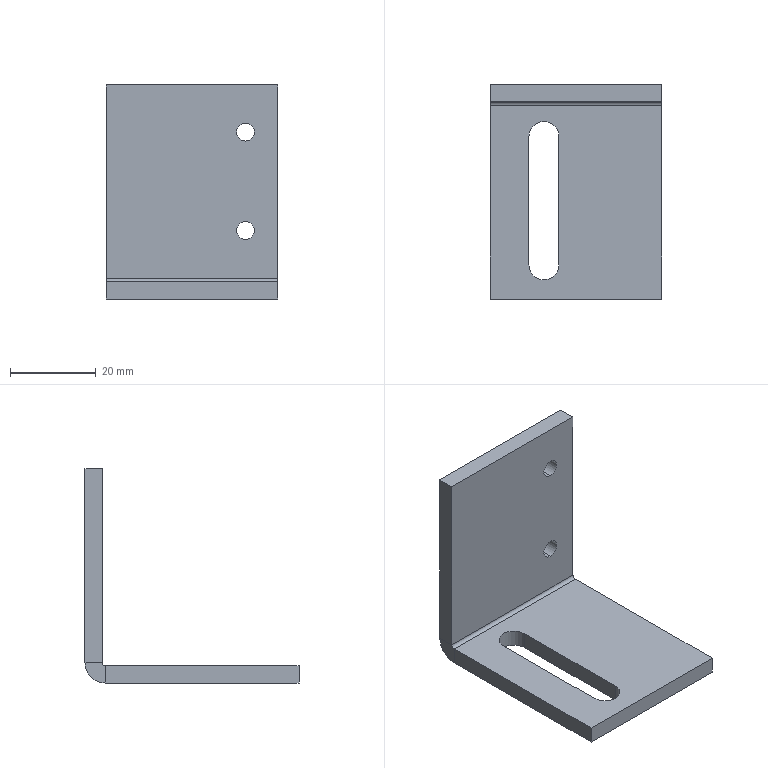Part | STEP file | drag chain fixing sheet metal_default | 1 solid | 22 faces | box 40 x 50 x 50 mm | volume 14067 mm3 | plane 14 | cylinder 8 | commonest cylinder face diameters 4.2 x4 7 x2 1.473 x1 9.473 x1